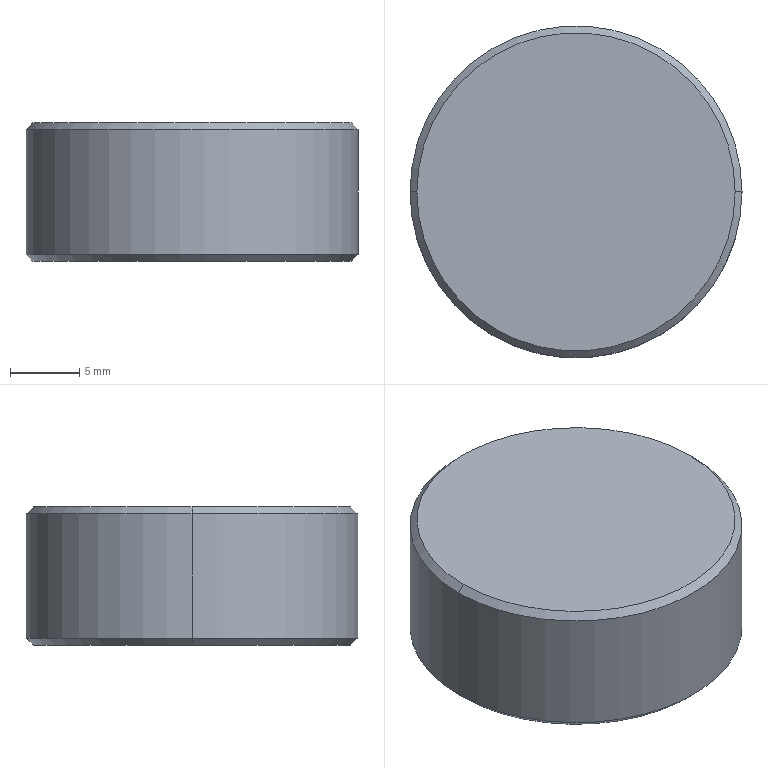Part | SolidWorks | features Chamfer 1, Extrusion 1, ICE 1 | 1 solid | 15 faces | box 24 x 24 x 10 mm | volume 4256 mm3 | plane 9 | cone 4 | cylinder 2 | commonest cylinder face diameters 24 x2
STEP:
#1=CARTESIAN_POINT('',(11.5,0.,10.));
#2=VERTEX_POINT('',#1);
#3=CARTESIAN_POINT('',(-11.5,0.,10.));
#4=VERTEX_POINT('',#3);
#5=CARTESIAN_POINT('',(0.,0.,10.));
#6=DIRECTION('',(0.,0.,1.));
#7=DIRECTION('',(1.,0.,0.));
#8=AXIS2_PLACEMENT_3D('',#5,#6,#7);
#9=CIRCLE('',#8,11.5);
#10=EDGE_CURVE('',#2,#4,#9,.T.);
#11=ORIENTED_EDGE('',*,*,#10,.F.);
#12=CARTESIAN_POINT('',(12.,0.,9.5));
#13=VERTEX_POINT('',#12);
#14=CARTESIAN_POINT('',(11.5,0.,10.));
#15=DIRECTION('',(0.7071,0.,-0.7071));
#16=VECTOR('',#15,1000.);
#17=LINE('',#14,#16);
#18=EDGE_CURVE('',#2,#13,#17,.T.);
#19=ORIENTED_EDGE('',*,*,#18,.T.);
#20=CARTESIAN_POINT('',(-12.,0.,9.5));
#21=VERTEX_POINT('',#20);
#22=CARTESIAN_POINT('',(0.,0.,9.5));
#23=DIRECTION('',(0.,0.,-1.));
#24=DIRECTION('',(1.,0.,0.));
#25=AXIS2_PLACEMENT_3D('',#22,#23,#24);
#26=CIRCLE('',#25,12.);
#27=EDGE_CURVE('',#21,#13,#26,.T.);
#28=ORIENTED_EDGE('',*,*,#27,.F.);
#29=CARTESIAN_POINT('',(-11.5,0.,10.));
#30=DIRECTION('',(-0.7071,0.,-0.7071));
#31=VECTOR('',#30,1000.);
#32=LINE('',#29,#31);
#33=EDGE_CURVE('',#4,#21,#32,.T.);
#34=ORIENTED_EDGE('',*,*,#33,.F.);
#35=EDGE_LOOP('',(#11,#19,#28,#34));
#36=FACE_OUTER_BOUND('',#35,.T.);
#37=CARTESIAN_POINT('',(0.,0.,10.));
#38=DIRECTION('',(0.,0.,-1.));
#39=DIRECTION('',(-1.,0.,0.));
#40=AXIS2_PLACEMENT_3D('',#37,#38,#39);
#41=CONICAL_SURFACE('',#40,11.5,0.7854);
#42=ADVANCED_FACE('',(#36),#41,.T.);
#43=CARTESIAN_POINT('',(-11.5,0.,0.));
#44=VERTEX_POINT('',#43);
#45=CARTESIAN_POINT('',(11.5,0.,0.));
#46=VERTEX_POINT('',#45);
#47=CARTESIAN_POINT('',(0.,0.,0.));
#48=DIRECTION('',(0.,0.,-1.));
#49=DIRECTION('',(1.,0.,0.));
#50=AXIS2_PLACEMENT_3D('',#47,#48,#49);
#51=CIRCLE('',#50,11.5);
#52=EDGE_CURVE('',#44,#46,#51,.T.);
#53=ORIENTED_EDGE('',*,*,#52,.F.);
#54=CARTESIAN_POINT('',(-12.,0.,0.5));
#55=VERTEX_POINT('',#54);
#56=CARTESIAN_POINT('',(-12.,0.,0.5));
#57=DIRECTION('',(-0.7071,0.,0.7071));
#58=VECTOR('',#57,1000.);
#59=LINE('',#56,#58);
#60=EDGE_CURVE('',#44,#55,#59,.T.);
#61=ORIENTED_EDGE('',*,*,#60,.T.);
#62=CARTESIAN_POINT('',(12.,0.,0.5));
#63=VERTEX_POINT('',#62);
#64=CARTESIAN_POINT('',(0.,0.,0.5));
#65=DIRECTION('',(0.,0.,1.));
#66=DIRECTION('',(1.,0.,0.));
#67=AXIS2_PLACEMENT_3D('',#64,#65,#66);
#68=CIRCLE('',#67,12.);
#69=EDGE_CURVE('',#63,#55,#68,.T.);
#70=ORIENTED_EDGE('',*,*,#69,.F.);
#71=CARTESIAN_POINT('',(12.,0.,0.5));
#72=DIRECTION('',(0.7071,0.,0.7071));
#73=VECTOR('',#72,1000.);
#74=LINE('',#71,#73);
#75=EDGE_CURVE('',#46,#63,#74,.T.);
#76=ORIENTED_EDGE('',*,*,#75,.F.);
#77=EDGE_LOOP('',(#53,#61,#70,#76));
#78=FACE_OUTER_BOUND('',#77,.T.);
#79=CARTESIAN_POINT('',(0.,0.,0.5));
#80=DIRECTION('',(0.,0.,1.));
#81=DIRECTION('',(1.,0.,0.));
#82=AXIS2_PLACEMENT_3D('',#79,#80,#81);
#83=CONICAL_SURFACE('',#82,12.,0.7854);
#84=ADVANCED_FACE('',(#78),#83,.T.);
#85=ORIENTED_EDGE('',*,*,#27,.T.);
#86=CARTESIAN_POINT('',(12.,0.,10.));
#87=DIRECTION('',(0.,0.,-1.));
#88=VECTOR('',#87,1000.);
#89=LINE('',#86,#88);
#90=EDGE_CURVE('',#13,#63,#89,.T.);
#91=ORIENTED_EDGE('',*,*,#90,.T.);
#92=ORIENTED_EDGE('',*,*,#69,.T.);
#93=CARTESIAN_POINT('',(-12.,0.,10.));
#94=DIRECTION('',(0.,0.,-1.));
#95=VECTOR('',#94,1000.);
#96=LINE('',#93,#95);
#97=EDGE_CURVE('',#21,#55,#96,.T.);
#98=ORIENTED_EDGE('',*,*,#97,.F.);
#99=EDGE_LOOP('',(#85,#91,#92,#98));
#100=FACE_OUTER_BOUND('',#99,.T.);
#101=CARTESIAN_POINT('',(0.,0.,10.));
#102=DIRECTION('',(0.,0.,-1.));
#103=DIRECTION('',(-1.,0.,0.));
#104=AXIS2_PLACEMENT_3D('',#101,#102,#103);
#105=CYLINDRICAL_SURFACE('',#104,12.);
#106=ADVANCED_FACE('',(#100),#105,.T.);
#107=ORIENTED_EDGE('',*,*,#90,.F.);
#108=CARTESIAN_POINT('',(0.,0.,9.5));
#109=DIRECTION('',(0.,0.,-1.));
#110=DIRECTION('',(1.,0.,0.));
#111=AXIS2_PLACEMENT_3D('',#108,#109,#110);
#112=CIRCLE('',#111,12.);
#113=EDGE_CURVE('',#13,#21,#112,.T.);
#114=ORIENTED_EDGE('',*,*,#113,.T.);
#115=ORIENTED_EDGE('',*,*,#97,.T.);
#116=CARTESIAN_POINT('',(0.,0.,0.5));
#117=DIRECTION('',(0.,0.,1.));
#118=DIRECTION('',(1.,0.,0.));
#119=AXIS2_PLACEMENT_3D('',#116,#117,#118);
#120=CIRCLE('',#119,12.);
#121=EDGE_CURVE('',#55,#63,#120,.T.);
#122=ORIENTED_EDGE('',*,*,#121,.T.);
#123=EDGE_LOOP('',(#107,#114,#115,#122));
#124=FACE_OUTER_BOUND('',#123,.T.);
#125=CARTESIAN_POINT('',(0.,0.,10.));
#126=DIRECTION('',(0.,0.,-1.));
#127=DIRECTION('',(-1.,0.,0.));
#128=AXIS2_PLACEMENT_3D('',#125,#126,#127);
#129=CYLINDRICAL_SURFACE('',#128,12.);
#130=ADVANCED_FACE('',(#124),#129,.T.);
#131=CARTESIAN_POINT('',(0.,0.,10.));
#132=DIRECTION('',(0.,0.,1.));
#133=DIRECTION('',(1.,0.,0.));
#134=AXIS2_PLACEMENT_3D('',#131,#132,#133);
#135=CIRCLE('',#134,11.5);
#136=EDGE_CURVE('',#4,#2,#135,.T.);
#137=ORIENTED_EDGE('',*,*,#136,.T.);
#138=ORIENTED_EDGE('',*,*,#10,.T.);
#139=EDGE_LOOP('',(#137,#138));
#140=FACE_OUTER_BOUND('',#139,.T.);
#141=CARTESIAN_POINT('',(0.,0.,10.));
#142=DIRECTION('',(0.,0.,1.));
#143=DIRECTION('',(1.,0.,0.));
#144=AXIS2_PLACEMENT_3D('',#141,#142,#143);
#145=PLANE('',#144);
#146=ADVANCED_FACE('',(#140),#145,.T.);
#147=CARTESIAN_POINT('',(0.,-3.464,0.));
#148=VERTEX_POINT('',#147);
#149=CARTESIAN_POINT('',(-3.,-1.732,0.));
#150=VERTEX_POINT('',#149);
#151=CARTESIAN_POINT('',(0.,-3.464,0.));
#152=DIRECTION('',(-0.866,0.5,0.));
#153=VECTOR('',#152,1000.);
#154=LINE('',#151,#153);
#155=EDGE_CURVE('',#148,#150,#154,.T.);
#156=ORIENTED_EDGE('',*,*,#155,.F.);
#157=CARTESIAN_POINT('',(3.,-1.732,0.));
#158=VERTEX_POINT('',#157);
#159=CARTESIAN_POINT('',(3.,-1.732,0.));
#160=DIRECTION('',(-0.866,-0.5,0.));
#161=VECTOR('',#160,1000.);
#162=LINE('',#159,#161);
#163=EDGE_CURVE('',#158,#148,#162,.T.);
#164=ORIENTED_EDGE('',*,*,#163,.F.);
#165=CARTESIAN_POINT('',(3.,1.732,0.));
#166=VERTEX_POINT('',#165);
#167=CARTESIAN_POINT('',(3.,1.732,0.));
#168=DIRECTION('',(0.,-1.,0.));
#169=VECTOR('',#168,1000.);
#170=LINE('',#167,#169);
#171=EDGE_CURVE('',#166,#158,#170,.T.);
#172=ORIENTED_EDGE('',*,*,#171,.F.);
#173=CARTESIAN_POINT('',(0.,3.464,0.));
#174=VERTEX_POINT('',#173);
#175=CARTESIAN_POINT('',(0.,3.464,0.));
#176=DIRECTION('',(0.866,-0.5,0.));
#177=VECTOR('',#176,1000.);
#178=LINE('',#175,#177);
#179=EDGE_CURVE('',#174,#166,#178,.T.);
#180=ORIENTED_EDGE('',*,*,#179,.F.);
#181=CARTESIAN_POINT('',(-3.,1.732,0.));
#182=VERTEX_POINT('',#181);
#183=CARTESIAN_POINT('',(-3.,1.732,0.));
#184=DIRECTION('',(0.866,0.5,0.));
#185=VECTOR('',#184,1000.);
#186=LINE('',#183,#185);
#187=EDGE_CURVE('',#182,#174,#186,.T.);
#188=ORIENTED_EDGE('',*,*,#187,.F.);
#189=CARTESIAN_POINT('',(-3.,-1.732,0.));
#190=DIRECTION('',(0.,1.,0.));
#191=VECTOR('',#190,1000.);
#192=LINE('',#189,#191);
#193=EDGE_CURVE('',#150,#182,#192,.T.);
#194=ORIENTED_EDGE('',*,*,#193,.F.);
#195=EDGE_LOOP('',(#156,#164,#172,#180,#188,#194));
#196=FACE_BOUND('',#195,.T.);
#197=CARTESIAN_POINT('',(0.,0.,0.));
#198=DIRECTION('',(0.,0.,-1.));
#199=DIRECTION('',(1.,0.,0.));
#200=AXIS2_PLACEMENT_3D('',#197,#198,#199);
#201=CIRCLE('',#200,11.5);
#202=EDGE_CURVE('',#46,#44,#201,.T.);
#203=ORIENTED_EDGE('',*,*,#202,.T.);
#204=ORIENTED_EDGE('',*,*,#52,.T.);
#205=EDGE_LOOP('',(#203,#204));
#206=FACE_OUTER_BOUND('',#205,.T.);
#207=CARTESIAN_POINT('',(0.,0.,0.));
#208=DIRECTION('',(0.,0.,1.));
#209=DIRECTION('',(1.,0.,0.));
#210=AXIS2_PLACEMENT_3D('',#207,#208,#209);
#211=PLANE('',#210);
#212=ADVANCED_FACE('',(#196,#206),#211,.F.);
#213=ORIENTED_EDGE('',*,*,#60,.F.);
#214=ORIENTED_EDGE('',*,*,#202,.F.);
#215=ORIENTED_EDGE('',*,*,#75,.T.);
#216=ORIENTED_EDGE('',*,*,#121,.F.);
#217=EDGE_LOOP('',(#213,#214,#215,#216));
#218=FACE_OUTER_BOUND('',#217,.T.);
#219=CARTESIAN_POINT('',(0.,0.,0.5));
#220=DIRECTION('',(0.,0.,1.));
#221=DIRECTION('',(1.,0.,0.));
#222=AXIS2_PLACEMENT_3D('',#219,#220,#221);
#223=CONICAL_SURFACE('',#222,12.,0.7854);
#224=ADVANCED_FACE('',(#218),#223,.T.);
#225=ORIENTED_EDGE('',*,*,#18,.F.);
#226=ORIENTED_EDGE('',*,*,#136,.F.);
#227=ORIENTED_EDGE('',*,*,#33,.T.);
#228=ORIENTED_EDGE('',*,*,#113,.F.);
#229=EDGE_LOOP('',(#225,#226,#227,#228));
#230=FACE_OUTER_BOUND('',#229,.T.);
#231=CARTESIAN_POINT('',(0.,0.,10.));
#232=DIRECTION('',(0.,0.,-1.));
#233=DIRECTION('',(-1.,0.,0.));
#234=AXIS2_PLACEMENT_3D('',#231,#232,#233);
#235=CONICAL_SURFACE('',#234,11.5,0.7854);
#236=ADVANCED_FACE('',(#230),#235,.T.);
#237=ORIENTED_EDGE('',*,*,#163,.T.);
#238=CARTESIAN_POINT('',(0.,-3.464,8.));
#239=VERTEX_POINT('',#238);
#240=CARTESIAN_POINT('',(0.,-3.464,8.));
#241=DIRECTION('',(0.,0.,-1.));
#242=VECTOR('',#241,1000.);
#243=LINE('',#240,#242);
#244=EDGE_CURVE('',#239,#148,#243,.T.);
#245=ORIENTED_EDGE('',*,*,#244,.F.);
#246=CARTESIAN_POINT('',(3.,-1.732,8.));
#247=VERTEX_POINT('',#246);
#248=CARTESIAN_POINT('',(3.,-1.732,8.));
#249=DIRECTION('',(-0.866,-0.5,0.));
#250=VECTOR('',#249,1000.);
#251=LINE('',#248,#250);
#252=EDGE_CURVE('',#247,#239,#251,.T.);
#253=ORIENTED_EDGE('',*,*,#252,.F.);
#254=CARTESIAN_POINT('',(3.,-1.732,8.));
#255=DIRECTION('',(0.,0.,-1.));
#256=VECTOR('',#255,1000.);
#257=LINE('',#254,#256);
#258=EDGE_CURVE('',#247,#158,#257,.T.);
#259=ORIENTED_EDGE('',*,*,#258,.T.);
#260=EDGE_LOOP('',(#237,#245,#253,#259));
#261=FACE_OUTER_BOUND('',#260,.T.);
#262=CARTESIAN_POINT('',(3.,-1.732,8.));
#263=DIRECTION('',(0.5,-0.866,0.));
#264=DIRECTION('',(0.866,0.5,0.));
#265=AXIS2_PLACEMENT_3D('',#262,#263,#264);
#266=PLANE('',#265);
#267=ADVANCED_FACE('',(#261),#266,.F.);
#268=ORIENTED_EDGE('',*,*,#171,.T.);
#269=ORIENTED_EDGE('',*,*,#258,.F.);
#270=CARTESIAN_POINT('',(3.,1.732,8.));
#271=VERTEX_POINT('',#270);
#272=CARTESIAN_POINT('',(3.,1.732,8.));
#273=DIRECTION('',(0.,-1.,0.));
#274=VECTOR('',#273,1000.);
#275=LINE('',#272,#274);
#276=EDGE_CURVE('',#271,#247,#275,.T.);
#277=ORIENTED_EDGE('',*,*,#276,.F.);
#278=CARTESIAN_POINT('',(3.,1.732,8.));
#279=DIRECTION('',(0.,0.,-1.));
#280=VECTOR('',#279,1000.);
#281=LINE('',#278,#280);
#282=EDGE_CURVE('',#271,#166,#281,.T.);
#283=ORIENTED_EDGE('',*,*,#282,.T.);
#284=EDGE_LOOP('',(#268,#269,#277,#283));
#285=FACE_OUTER_BOUND('',#284,.T.);
#286=CARTESIAN_POINT('',(3.,1.732,8.));
#287=DIRECTION('',(1.,0.,0.));
#288=DIRECTION('',(0.,1.,0.));
#289=AXIS2_PLACEMENT_3D('',#286,#287,#288);
#290=PLANE('',#289);
#291=ADVANCED_FACE('',(#285),#290,.F.);
#292=ORIENTED_EDGE('',*,*,#179,.T.);
#293=ORIENTED_EDGE('',*,*,#282,.F.);
#294=CARTESIAN_POINT('',(0.,3.464,8.));
#295=VERTEX_POINT('',#294);
#296=CARTESIAN_POINT('',(0.,3.464,8.));
#297=DIRECTION('',(0.866,-0.5,0.));
#298=VECTOR('',#297,1000.);
#299=LINE('',#296,#298);
#300=EDGE_CURVE('',#295,#271,#299,.T.);
#301=ORIENTED_EDGE('',*,*,#300,.F.);
#302=CARTESIAN_POINT('',(0.,3.464,8.));
#303=DIRECTION('',(0.,0.,-1.));
#304=VECTOR('',#303,1000.);
#305=LINE('',#302,#304);
#306=EDGE_CURVE('',#295,#174,#305,.T.);
#307=ORIENTED_EDGE('',*,*,#306,.T.);
#308=EDGE_LOOP('',(#292,#293,#301,#307));
#309=FACE_OUTER_BOUND('',#308,.T.);
#310=CARTESIAN_POINT('',(0.,3.464,8.));
#311=DIRECTION('',(0.5,0.866,0.));
#312=DIRECTION('',(-0.866,0.5,0.));
#313=AXIS2_PLACEMENT_3D('',#310,#311,#312);
#314=PLANE('',#313);
#315=ADVANCED_FACE('',(#309),#314,.F.);
#316=ORIENTED_EDGE('',*,*,#187,.T.);
#317=ORIENTED_EDGE('',*,*,#306,.F.);
#318=CARTESIAN_POINT('',(-3.,1.732,8.));
#319=VERTEX_POINT('',#318);
#320=CARTESIAN_POINT('',(-3.,1.732,8.));
#321=DIRECTION('',(0.866,0.5,0.));
#322=VECTOR('',#321,1000.);
#323=LINE('',#320,#322);
#324=EDGE_CURVE('',#319,#295,#323,.T.);
#325=ORIENTED_EDGE('',*,*,#324,.F.);
#326=CARTESIAN_POINT('',(-3.,1.732,8.));
#327=DIRECTION('',(0.,0.,-1.));
#328=VECTOR('',#327,1000.);
#329=LINE('',#326,#328);
#330=EDGE_CURVE('',#319,#182,#329,.T.);
#331=ORIENTED_EDGE('',*,*,#330,.T.);
#332=EDGE_LOOP('',(#316,#317,#325,#331));
#333=FACE_OUTER_BOUND('',#332,.T.);
#334=CARTESIAN_POINT('',(-3.,1.732,8.));
#335=DIRECTION('',(-0.5,0.866,0.));
#336=DIRECTION('',(-0.866,-0.5,0.));
#337=AXIS2_PLACEMENT_3D('',#334,#335,#336);
#338=PLANE('',#337);
#339=ADVANCED_FACE('',(#333),#338,.F.);
#340=ORIENTED_EDGE('',*,*,#193,.T.);
#341=ORIENTED_EDGE('',*,*,#330,.F.);
#342=CARTESIAN_POINT('',(-3.,-1.732,8.));
#343=VERTEX_POINT('',#342);
#344=CARTESIAN_POINT('',(-3.,-1.732,8.));
#345=DIRECTION('',(0.,1.,0.));
#346=VECTOR('',#345,1000.);
#347=LINE('',#344,#346);
#348=EDGE_CURVE('',#343,#319,#347,.T.);
#349=ORIENTED_EDGE('',*,*,#348,.F.);
#350=CARTESIAN_POINT('',(-3.,-1.732,8.));
#351=DIRECTION('',(0.,0.,-1.));
#352=VECTOR('',#351,1000.);
#353=LINE('',#350,#352);
#354=EDGE_CURVE('',#343,#150,#353,.T.);
#355=ORIENTED_EDGE('',*,*,#354,.T.);
#356=EDGE_LOOP('',(#340,#341,#349,#355));
#357=FACE_OUTER_BOUND('',#356,.T.);
#358=CARTESIAN_POINT('',(-3.,-1.732,8.));
#359=DIRECTION('',(-1.,0.,0.));
#360=DIRECTION('',(0.,0.,1.));
#361=AXIS2_PLACEMENT_3D('',#358,#359,#360);
#362=PLANE('',#361);
#363=ADVANCED_FACE('',(#357),#362,.F.);
#364=ORIENTED_EDGE('',*,*,#155,.T.);
#365=ORIENTED_EDGE('',*,*,#354,.F.);
#366=CARTESIAN_POINT('',(0.,-3.464,8.));
#367=DIRECTION('',(-0.866,0.5,0.));
#368=VECTOR('',#367,1000.);
#369=LINE('',#366,#368);
#370=EDGE_CURVE('',#239,#343,#369,.T.);
#371=ORIENTED_EDGE('',*,*,#370,.F.);
#372=ORIENTED_EDGE('',*,*,#244,.T.);
#373=EDGE_LOOP('',(#364,#365,#371,#372));
#374=FACE_OUTER_BOUND('',#373,.T.);
#375=CARTESIAN_POINT('',(0.,-3.464,8.));
#376=DIRECTION('',(-0.5,-0.866,0.));
#377=DIRECTION('',(0.866,-0.5,0.));
#378=AXIS2_PLACEMENT_3D('',#375,#376,#377);
#379=PLANE('',#378);
#380=ADVANCED_FACE('',(#374),#379,.F.);
#381=ORIENTED_EDGE('',*,*,#252,.T.);
#382=ORIENTED_EDGE('',*,*,#370,.T.);
#383=ORIENTED_EDGE('',*,*,#348,.T.);
#384=ORIENTED_EDGE('',*,*,#324,.T.);
#385=ORIENTED_EDGE('',*,*,#300,.T.);
#386=ORIENTED_EDGE('',*,*,#276,.T.);
#387=EDGE_LOOP('',(#381,#382,#383,#384,#385,#386));
#388=FACE_OUTER_BOUND('',#387,.T.);
#389=CARTESIAN_POINT('',(0.,0.,8.));
#390=DIRECTION('',(0.,0.,-1.));
#391=DIRECTION('',(-1.,0.,0.));
#392=AXIS2_PLACEMENT_3D('',#389,#390,#391);
#393=PLANE('',#392);
#394=ADVANCED_FACE('',(#388),#393,.T.);
#395=CLOSED_SHELL('',(#42,#84,#106,#130,#146,#212,#224,#236,#267,#291,#315,#339,#363,#380,#394));
#396=MANIFOLD_SOLID_BREP('',#395);
#397=CARTESIAN_POINT('',(0.,0.,0.));
#398=DIRECTION('',(0.,0.,1.));
#399=DIRECTION('',(1.,0.,0.));
#400=AXIS2_PLACEMENT_3D('',#397,#398,#399);
#401=(LENGTH_UNIT()NAMED_UNIT(*)SI_UNIT(.MILLI.,.METRE.));
#402=UNCERTAINTY_MEASURE_WITH_UNIT(LENGTH_MEASURE(0.00001),#401,'','');
#403=(NAMED_UNIT(*)PLANE_ANGLE_UNIT()SI_UNIT($,.RADIAN.));
#404=(NAMED_UNIT(*)SI_UNIT($,.STERADIAN.)SOLID_ANGLE_UNIT());
#405=(GEOMETRIC_REPRESENTATION_CONTEXT(3)GLOBAL_UNCERTAINTY_ASSIGNED_CONTEXT((#402))GLOBAL_UNIT_ASSIGNED_CONTEXT((#401,#403,#404))REPRESENTATION_CONTEXT('',''));
#406=ADVANCED_BREP_SHAPE_REPRESENTATION('',(#396,#400),#405);